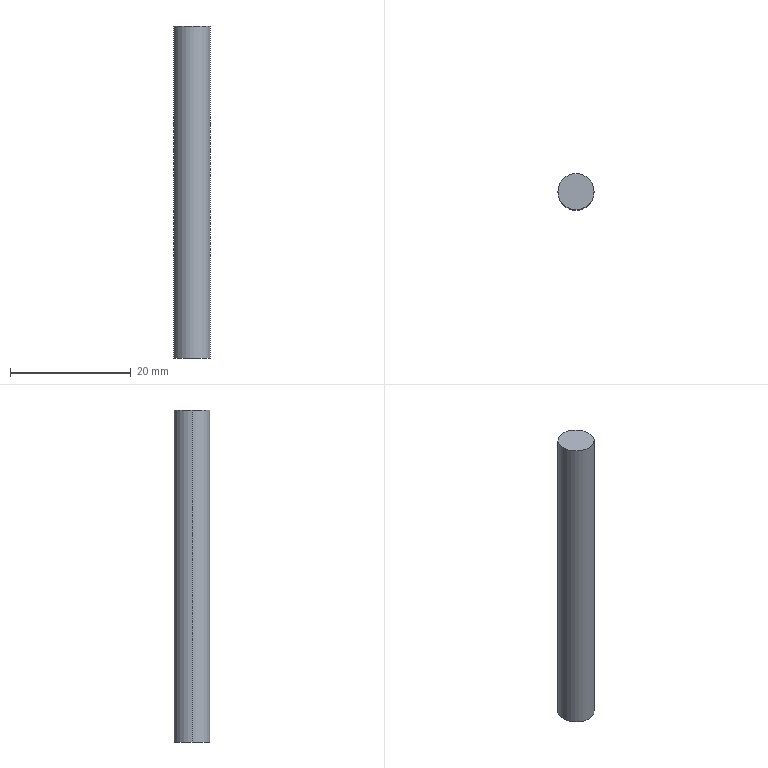Part | SolidWorks | features Extrusion 1 | 1 solid | 4 faces | box 6 x 6 x 55 mm | volume 1555 mm3 | cylinder 2 | plane 2 | commonest cylinder face diameters 6 x2
STEP:
#1=CARTESIAN_POINT('',(3.,0.,55.));
#2=VERTEX_POINT('',#1);
#3=CARTESIAN_POINT('',(-3.,0.,55.));
#4=VERTEX_POINT('',#3);
#5=CARTESIAN_POINT('',(0.,0.,55.));
#6=DIRECTION('',(0.,0.,1.));
#7=DIRECTION('',(1.,0.,0.));
#8=AXIS2_PLACEMENT_3D('',#5,#6,#7);
#9=CIRCLE('',#8,3.);
#10=EDGE_CURVE('',#2,#4,#9,.T.);
#11=ORIENTED_EDGE('',*,*,#10,.F.);
#12=CARTESIAN_POINT('',(3.,0.,0.));
#13=VERTEX_POINT('',#12);
#14=CARTESIAN_POINT('',(3.,0.,55.));
#15=DIRECTION('',(0.,0.,-1.));
#16=VECTOR('',#15,1000.);
#17=LINE('',#14,#16);
#18=EDGE_CURVE('',#2,#13,#17,.T.);
#19=ORIENTED_EDGE('',*,*,#18,.T.);
#20=CARTESIAN_POINT('',(-3.,0.,0.));
#21=VERTEX_POINT('',#20);
#22=CARTESIAN_POINT('',(0.,0.,0.));
#23=DIRECTION('',(0.,0.,1.));
#24=DIRECTION('',(1.,0.,0.));
#25=AXIS2_PLACEMENT_3D('',#22,#23,#24);
#26=CIRCLE('',#25,3.);
#27=EDGE_CURVE('',#13,#21,#26,.T.);
#28=ORIENTED_EDGE('',*,*,#27,.T.);
#29=CARTESIAN_POINT('',(-3.,0.,55.));
#30=DIRECTION('',(0.,0.,-1.));
#31=VECTOR('',#30,1000.);
#32=LINE('',#29,#31);
#33=EDGE_CURVE('',#4,#21,#32,.T.);
#34=ORIENTED_EDGE('',*,*,#33,.F.);
#35=EDGE_LOOP('',(#11,#19,#28,#34));
#36=FACE_OUTER_BOUND('',#35,.T.);
#37=CARTESIAN_POINT('',(0.,0.,55.));
#38=DIRECTION('',(0.,0.,-1.));
#39=DIRECTION('',(-1.,0.,0.));
#40=AXIS2_PLACEMENT_3D('',#37,#38,#39);
#41=CYLINDRICAL_SURFACE('',#40,3.);
#42=ADVANCED_FACE('',(#36),#41,.T.);
#43=ORIENTED_EDGE('',*,*,#18,.F.);
#44=CARTESIAN_POINT('',(0.,0.,55.));
#45=DIRECTION('',(0.,0.,1.));
#46=DIRECTION('',(1.,0.,0.));
#47=AXIS2_PLACEMENT_3D('',#44,#45,#46);
#48=CIRCLE('',#47,3.);
#49=EDGE_CURVE('',#4,#2,#48,.T.);
#50=ORIENTED_EDGE('',*,*,#49,.F.);
#51=ORIENTED_EDGE('',*,*,#33,.T.);
#52=CARTESIAN_POINT('',(0.,0.,0.));
#53=DIRECTION('',(0.,0.,1.));
#54=DIRECTION('',(1.,0.,0.));
#55=AXIS2_PLACEMENT_3D('',#52,#53,#54);
#56=CIRCLE('',#55,3.);
#57=EDGE_CURVE('',#21,#13,#56,.T.);
#58=ORIENTED_EDGE('',*,*,#57,.T.);
#59=EDGE_LOOP('',(#43,#50,#51,#58));
#60=FACE_OUTER_BOUND('',#59,.T.);
#61=CARTESIAN_POINT('',(0.,0.,55.));
#62=DIRECTION('',(0.,0.,-1.));
#63=DIRECTION('',(-1.,0.,0.));
#64=AXIS2_PLACEMENT_3D('',#61,#62,#63);
#65=CYLINDRICAL_SURFACE('',#64,3.);
#66=ADVANCED_FACE('',(#60),#65,.T.);
#67=ORIENTED_EDGE('',*,*,#49,.T.);
#68=ORIENTED_EDGE('',*,*,#10,.T.);
#69=EDGE_LOOP('',(#67,#68));
#70=FACE_OUTER_BOUND('',#69,.T.);
#71=CARTESIAN_POINT('',(0.,0.,55.));
#72=DIRECTION('',(0.,0.,1.));
#73=DIRECTION('',(1.,0.,0.));
#74=AXIS2_PLACEMENT_3D('',#71,#72,#73);
#75=PLANE('',#74);
#76=ADVANCED_FACE('',(#70),#75,.T.);
#77=ORIENTED_EDGE('',*,*,#57,.F.);
#78=ORIENTED_EDGE('',*,*,#27,.F.);
#79=EDGE_LOOP('',(#77,#78));
#80=FACE_OUTER_BOUND('',#79,.T.);
#81=CARTESIAN_POINT('',(0.,0.,0.));
#82=DIRECTION('',(0.,0.,1.));
#83=DIRECTION('',(1.,0.,0.));
#84=AXIS2_PLACEMENT_3D('',#81,#82,#83);
#85=PLANE('',#84);
#86=ADVANCED_FACE('',(#80),#85,.F.);
#87=CLOSED_SHELL('',(#42,#66,#76,#86));
#88=MANIFOLD_SOLID_BREP('',#87);
#89=CARTESIAN_POINT('',(0.,0.,0.));
#90=DIRECTION('',(0.,0.,1.));
#91=DIRECTION('',(1.,0.,0.));
#92=AXIS2_PLACEMENT_3D('',#89,#90,#91);
#93=(LENGTH_UNIT()NAMED_UNIT(*)SI_UNIT(.MILLI.,.METRE.));
#94=UNCERTAINTY_MEASURE_WITH_UNIT(LENGTH_MEASURE(0.00001),#93,'','');
#95=(NAMED_UNIT(*)PLANE_ANGLE_UNIT()SI_UNIT($,.RADIAN.));
#96=(NAMED_UNIT(*)SI_UNIT($,.STERADIAN.)SOLID_ANGLE_UNIT());
#97=(GEOMETRIC_REPRESENTATION_CONTEXT(3)GLOBAL_UNCERTAINTY_ASSIGNED_CONTEXT((#94))GLOBAL_UNIT_ASSIGNED_CONTEXT((#93,#95,#96))REPRESENTATION_CONTEXT('',''));
#98=ADVANCED_BREP_SHAPE_REPRESENTATION('',(#88,#92),#97);